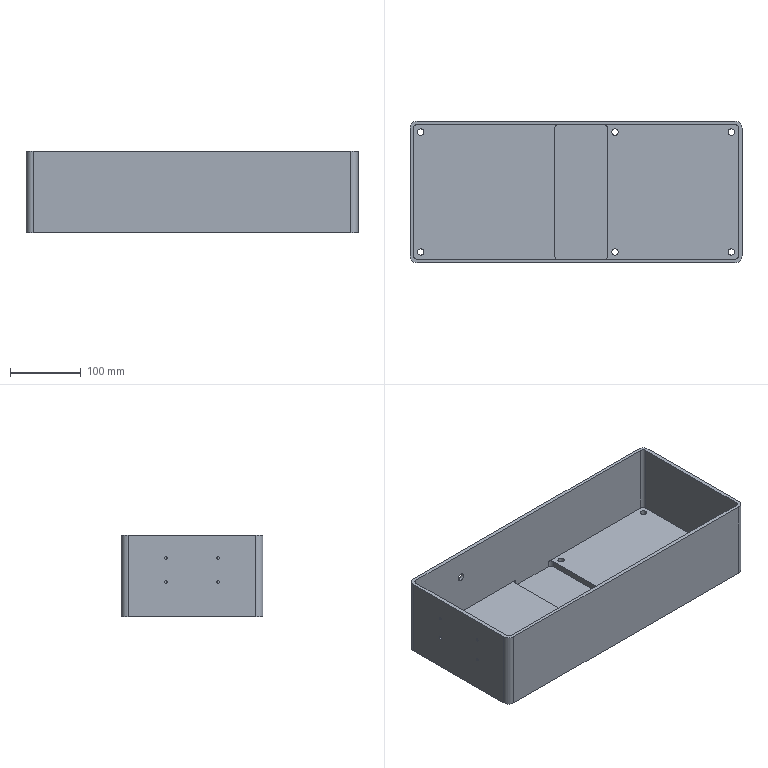Part | SolidWorks | features ICE 4, Fillet 3, Extrusion 1, HoleWzd 1, Shell 1 | 1 solid | 67 faces | box 470.5 x 201 x 115 mm | volume 1931028 mm3 | cylinder 46 | plane 21 | commonest cylinder face diameters 9 x12 15 x12 4.1 x8 10 x8 20 x4 11 x2